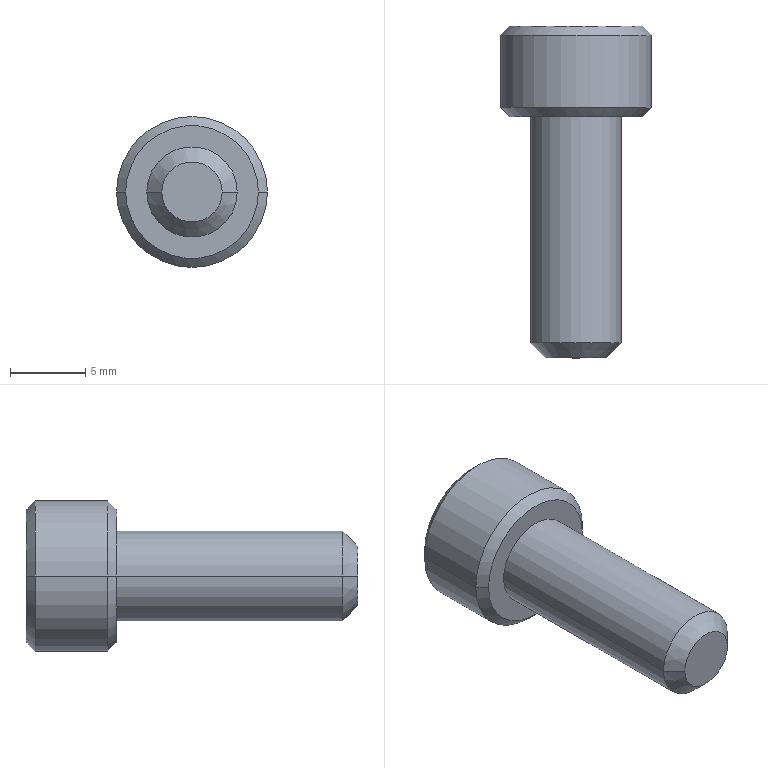Part | STEP file | BB62-M6-16L | 1 solid | 27 faces | box 10 x 22 x 10 mm | volume 826.496 mm3 | plane 15 | cone 8 | cylinder 4 | commonest cylinder face diameters 6 x2 10 x2